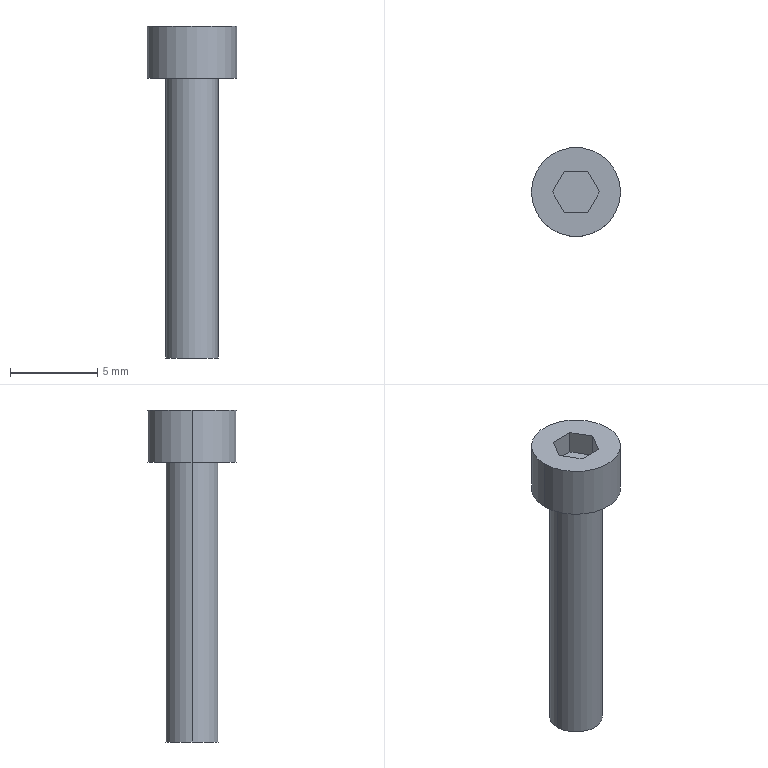Part | SolidWorks | features BaseBody 1 | 1 solid | 14 faces | box 5.1 x 5.1 x 19 mm | volume 167.99 mm3 | plane 10 | cylinder 4 | commonest cylinder face diameters 3 x2 5.1 x2
STEP:
#1=CARTESIAN_POINT('',(1.5,0.,-16.));
#2=VERTEX_POINT('',#1);
#3=CARTESIAN_POINT('',(-1.5,0.,-16.));
#4=VERTEX_POINT('',#3);
#5=CARTESIAN_POINT('',(0.,0.,-16.));
#6=DIRECTION('',(0.,0.,1.));
#7=DIRECTION('',(1.,0.,0.));
#8=AXIS2_PLACEMENT_3D('',#5,#6,#7);
#9=CIRCLE('',#8,1.5);
#10=EDGE_CURVE('',#2,#4,#9,.T.);
#11=ORIENTED_EDGE('',*,*,#10,.T.);
#12=CARTESIAN_POINT('',(-1.5,0.,0.));
#13=VERTEX_POINT('',#12);
#14=CARTESIAN_POINT('',(-1.5,0.,-16.));
#15=DIRECTION('',(0.,0.,1.));
#16=VECTOR('',#15,1000.);
#17=LINE('',#14,#16);
#18=EDGE_CURVE('',#4,#13,#17,.T.);
#19=ORIENTED_EDGE('',*,*,#18,.T.);
#20=CARTESIAN_POINT('',(1.5,0.,0.));
#21=VERTEX_POINT('',#20);
#22=CARTESIAN_POINT('',(0.,0.,0.));
#23=DIRECTION('',(0.,0.,-1.));
#24=DIRECTION('',(1.,0.,0.));
#25=AXIS2_PLACEMENT_3D('',#22,#23,#24);
#26=CIRCLE('',#25,1.5);
#27=EDGE_CURVE('',#13,#21,#26,.T.);
#28=ORIENTED_EDGE('',*,*,#27,.T.);
#29=CARTESIAN_POINT('',(1.5,0.,-16.));
#30=DIRECTION('',(0.,0.,1.));
#31=VECTOR('',#30,1000.);
#32=LINE('',#29,#31);
#33=EDGE_CURVE('',#2,#21,#32,.T.);
#34=ORIENTED_EDGE('',*,*,#33,.F.);
#35=EDGE_LOOP('',(#11,#19,#28,#34));
#36=FACE_OUTER_BOUND('',#35,.T.);
#37=CARTESIAN_POINT('',(0.,0.,-16.));
#38=DIRECTION('',(0.,0.,1.));
#39=DIRECTION('',(1.,0.,0.));
#40=AXIS2_PLACEMENT_3D('',#37,#38,#39);
#41=CYLINDRICAL_SURFACE('',#40,1.5);
#42=ADVANCED_FACE('',(#36),#41,.T.);
#43=CARTESIAN_POINT('',(2.55,0.,0.));
#44=VERTEX_POINT('',#43);
#45=CARTESIAN_POINT('',(-2.55,0.,0.));
#46=VERTEX_POINT('',#45);
#47=CARTESIAN_POINT('',(0.,0.,0.));
#48=DIRECTION('',(0.,0.,1.));
#49=DIRECTION('',(1.,0.,0.));
#50=AXIS2_PLACEMENT_3D('',#47,#48,#49);
#51=CIRCLE('',#50,2.55);
#52=EDGE_CURVE('',#44,#46,#51,.T.);
#53=ORIENTED_EDGE('',*,*,#52,.T.);
#54=CARTESIAN_POINT('',(-2.55,0.,3.));
#55=VERTEX_POINT('',#54);
#56=CARTESIAN_POINT('',(-2.55,0.,0.));
#57=DIRECTION('',(0.,0.,1.));
#58=VECTOR('',#57,1000.);
#59=LINE('',#56,#58);
#60=EDGE_CURVE('',#46,#55,#59,.T.);
#61=ORIENTED_EDGE('',*,*,#60,.T.);
#62=CARTESIAN_POINT('',(2.55,0.,3.));
#63=VERTEX_POINT('',#62);
#64=CARTESIAN_POINT('',(0.,0.,3.));
#65=DIRECTION('',(0.,0.,-1.));
#66=DIRECTION('',(1.,0.,0.));
#67=AXIS2_PLACEMENT_3D('',#64,#65,#66);
#68=CIRCLE('',#67,2.55);
#69=EDGE_CURVE('',#55,#63,#68,.T.);
#70=ORIENTED_EDGE('',*,*,#69,.T.);
#71=CARTESIAN_POINT('',(2.55,0.,0.));
#72=DIRECTION('',(0.,0.,1.));
#73=VECTOR('',#72,1000.);
#74=LINE('',#71,#73);
#75=EDGE_CURVE('',#44,#63,#74,.T.);
#76=ORIENTED_EDGE('',*,*,#75,.F.);
#77=EDGE_LOOP('',(#53,#61,#70,#76));
#78=FACE_OUTER_BOUND('',#77,.T.);
#79=CARTESIAN_POINT('',(0.,0.,0.));
#80=DIRECTION('',(0.,0.,1.));
#81=DIRECTION('',(1.,0.,0.));
#82=AXIS2_PLACEMENT_3D('',#79,#80,#81);
#83=CYLINDRICAL_SURFACE('',#82,2.55);
#84=ADVANCED_FACE('',(#78),#83,.T.);
#85=ORIENTED_EDGE('',*,*,#18,.F.);
#86=CARTESIAN_POINT('',(0.,0.,-16.));
#87=DIRECTION('',(0.,0.,1.));
#88=DIRECTION('',(1.,0.,0.));
#89=AXIS2_PLACEMENT_3D('',#86,#87,#88);
#90=CIRCLE('',#89,1.5);
#91=EDGE_CURVE('',#4,#2,#90,.T.);
#92=ORIENTED_EDGE('',*,*,#91,.T.);
#93=ORIENTED_EDGE('',*,*,#33,.T.);
#94=CARTESIAN_POINT('',(0.,0.,0.));
#95=DIRECTION('',(0.,0.,-1.));
#96=DIRECTION('',(1.,0.,0.));
#97=AXIS2_PLACEMENT_3D('',#94,#95,#96);
#98=CIRCLE('',#97,1.5);
#99=EDGE_CURVE('',#21,#13,#98,.T.);
#100=ORIENTED_EDGE('',*,*,#99,.T.);
#101=EDGE_LOOP('',(#85,#92,#93,#100));
#102=FACE_OUTER_BOUND('',#101,.T.);
#103=CARTESIAN_POINT('',(0.,0.,-16.));
#104=DIRECTION('',(0.,0.,1.));
#105=DIRECTION('',(1.,0.,0.));
#106=AXIS2_PLACEMENT_3D('',#103,#104,#105);
#107=CYLINDRICAL_SURFACE('',#106,1.5);
#108=ADVANCED_FACE('',(#102),#107,.T.);
#109=ORIENTED_EDGE('',*,*,#10,.F.);
#110=ORIENTED_EDGE('',*,*,#91,.F.);
#111=EDGE_LOOP('',(#109,#110));
#112=FACE_OUTER_BOUND('',#111,.T.);
#113=CARTESIAN_POINT('',(0.,0.,-16.));
#114=DIRECTION('',(0.,0.,1.));
#115=DIRECTION('',(1.,0.,0.));
#116=AXIS2_PLACEMENT_3D('',#113,#114,#115);
#117=PLANE('',#116);
#118=ADVANCED_FACE('',(#112),#117,.F.);
#119=ORIENTED_EDGE('',*,*,#99,.F.);
#120=ORIENTED_EDGE('',*,*,#27,.F.);
#121=EDGE_LOOP('',(#119,#120));
#122=FACE_BOUND('',#121,.T.);
#123=ORIENTED_EDGE('',*,*,#52,.F.);
#124=CARTESIAN_POINT('',(0.,0.,0.));
#125=DIRECTION('',(0.,0.,1.));
#126=DIRECTION('',(1.,0.,0.));
#127=AXIS2_PLACEMENT_3D('',#124,#125,#126);
#128=CIRCLE('',#127,2.55);
#129=EDGE_CURVE('',#46,#44,#128,.T.);
#130=ORIENTED_EDGE('',*,*,#129,.F.);
#131=EDGE_LOOP('',(#123,#130));
#132=FACE_OUTER_BOUND('',#131,.T.);
#133=CARTESIAN_POINT('',(0.,0.,0.));
#134=DIRECTION('',(0.,0.,1.));
#135=DIRECTION('',(1.,0.,0.));
#136=AXIS2_PLACEMENT_3D('',#133,#134,#135);
#137=PLANE('',#136);
#138=ADVANCED_FACE('',(#122,#132),#137,.F.);
#139=ORIENTED_EDGE('',*,*,#60,.F.);
#140=ORIENTED_EDGE('',*,*,#129,.T.);
#141=ORIENTED_EDGE('',*,*,#75,.T.);
#142=CARTESIAN_POINT('',(0.,0.,3.));
#143=DIRECTION('',(0.,0.,-1.));
#144=DIRECTION('',(1.,0.,0.));
#145=AXIS2_PLACEMENT_3D('',#142,#143,#144);
#146=CIRCLE('',#145,2.55);
#147=EDGE_CURVE('',#63,#55,#146,.T.);
#148=ORIENTED_EDGE('',*,*,#147,.T.);
#149=EDGE_LOOP('',(#139,#140,#141,#148));
#150=FACE_OUTER_BOUND('',#149,.T.);
#151=CARTESIAN_POINT('',(0.,0.,0.));
#152=DIRECTION('',(0.,0.,1.));
#153=DIRECTION('',(1.,0.,0.));
#154=AXIS2_PLACEMENT_3D('',#151,#152,#153);
#155=CYLINDRICAL_SURFACE('',#154,2.55);
#156=ADVANCED_FACE('',(#150),#155,.T.);
#157=CARTESIAN_POINT('',(-0.675,-1.169,3.));
#158=VERTEX_POINT('',#157);
#159=CARTESIAN_POINT('',(-1.35,0.,3.));
#160=VERTEX_POINT('',#159);
#161=CARTESIAN_POINT('',(-0.675,-1.169,3.));
#162=DIRECTION('',(-0.5,0.866,0.));
#163=VECTOR('',#162,1000.);
#164=LINE('',#161,#163);
#165=EDGE_CURVE('',#158,#160,#164,.T.);
#166=ORIENTED_EDGE('',*,*,#165,.T.);
#167=CARTESIAN_POINT('',(-0.675,1.169,3.));
#168=VERTEX_POINT('',#167);
#169=CARTESIAN_POINT('',(-1.35,0.,3.));
#170=DIRECTION('',(0.5,0.866,0.));
#171=VECTOR('',#170,1000.);
#172=LINE('',#169,#171);
#173=EDGE_CURVE('',#160,#168,#172,.T.);
#174=ORIENTED_EDGE('',*,*,#173,.T.);
#175=CARTESIAN_POINT('',(0.675,1.169,3.));
#176=VERTEX_POINT('',#175);
#177=CARTESIAN_POINT('',(0.,1.169,3.));
#178=DIRECTION('',(1.,0.,0.));
#179=VECTOR('',#178,1000.);
#180=LINE('',#177,#179);
#181=EDGE_CURVE('',#168,#176,#180,.T.);
#182=ORIENTED_EDGE('',*,*,#181,.T.);
#183=CARTESIAN_POINT('',(1.35,0.,3.));
#184=VERTEX_POINT('',#183);
#185=CARTESIAN_POINT('',(0.675,1.169,3.));
#186=DIRECTION('',(0.5,-0.866,0.));
#187=VECTOR('',#186,1000.);
#188=LINE('',#185,#187);
#189=EDGE_CURVE('',#176,#184,#188,.T.);
#190=ORIENTED_EDGE('',*,*,#189,.T.);
#191=CARTESIAN_POINT('',(0.675,-1.169,3.));
#192=VERTEX_POINT('',#191);
#193=CARTESIAN_POINT('',(1.35,0.,3.));
#194=DIRECTION('',(-0.5,-0.866,0.));
#195=VECTOR('',#194,1000.);
#196=LINE('',#193,#195);
#197=EDGE_CURVE('',#184,#192,#196,.T.);
#198=ORIENTED_EDGE('',*,*,#197,.T.);
#199=CARTESIAN_POINT('',(0.,-1.169,3.));
#200=DIRECTION('',(-1.,0.,0.));
#201=VECTOR('',#200,1000.);
#202=LINE('',#199,#201);
#203=EDGE_CURVE('',#192,#158,#202,.T.);
#204=ORIENTED_EDGE('',*,*,#203,.T.);
#205=EDGE_LOOP('',(#166,#174,#182,#190,#198,#204));
#206=FACE_BOUND('',#205,.T.);
#207=ORIENTED_EDGE('',*,*,#147,.F.);
#208=ORIENTED_EDGE('',*,*,#69,.F.);
#209=EDGE_LOOP('',(#207,#208));
#210=FACE_OUTER_BOUND('',#209,.T.);
#211=CARTESIAN_POINT('',(0.,0.,3.));
#212=DIRECTION('',(0.,0.,1.));
#213=DIRECTION('',(1.,0.,0.));
#214=AXIS2_PLACEMENT_3D('',#211,#212,#213);
#215=PLANE('',#214);
#216=ADVANCED_FACE('',(#206,#210),#215,.T.);
#217=ORIENTED_EDGE('',*,*,#173,.F.);
#218=CARTESIAN_POINT('',(-1.35,0.,1.65));
#219=VERTEX_POINT('',#218);
#220=CARTESIAN_POINT('',(-1.35,0.,1.65));
#221=DIRECTION('',(0.,0.,-1.));
#222=VECTOR('',#221,1000.);
#223=LINE('',#220,#222);
#224=EDGE_CURVE('',#160,#219,#223,.T.);
#225=ORIENTED_EDGE('',*,*,#224,.T.);
#226=CARTESIAN_POINT('',(-0.675,1.169,1.65));
#227=VERTEX_POINT('',#226);
#228=CARTESIAN_POINT('',(-0.675,1.169,1.65));
#229=DIRECTION('',(0.5,0.866,0.));
#230=VECTOR('',#229,1000.);
#231=LINE('',#228,#230);
#232=EDGE_CURVE('',#219,#227,#231,.T.);
#233=ORIENTED_EDGE('',*,*,#232,.T.);
#234=CARTESIAN_POINT('',(-0.675,1.169,1.65));
#235=DIRECTION('',(0.,0.,1.));
#236=VECTOR('',#235,1000.);
#237=LINE('',#234,#236);
#238=EDGE_CURVE('',#227,#168,#237,.T.);
#239=ORIENTED_EDGE('',*,*,#238,.T.);
#240=EDGE_LOOP('',(#217,#225,#233,#239));
#241=FACE_OUTER_BOUND('',#240,.T.);
#242=CARTESIAN_POINT('',(-0.675,1.169,1.65));
#243=DIRECTION('',(0.866,-0.5,0.));
#244=DIRECTION('',(0.5,0.866,0.));
#245=AXIS2_PLACEMENT_3D('',#242,#243,#244);
#246=PLANE('',#245);
#247=ADVANCED_FACE('',(#241),#246,.T.);
#248=ORIENTED_EDGE('',*,*,#165,.F.);
#249=CARTESIAN_POINT('',(-0.675,-1.169,1.65));
#250=VERTEX_POINT('',#249);
#251=CARTESIAN_POINT('',(-0.675,-1.169,1.65));
#252=DIRECTION('',(0.,0.,-1.));
#253=VECTOR('',#252,1000.);
#254=LINE('',#251,#253);
#255=EDGE_CURVE('',#158,#250,#254,.T.);
#256=ORIENTED_EDGE('',*,*,#255,.T.);
#257=CARTESIAN_POINT('',(-1.35,0.,1.65));
#258=DIRECTION('',(-0.5,0.866,0.));
#259=VECTOR('',#258,1000.);
#260=LINE('',#257,#259);
#261=EDGE_CURVE('',#250,#219,#260,.T.);
#262=ORIENTED_EDGE('',*,*,#261,.T.);
#263=ORIENTED_EDGE('',*,*,#224,.F.);
#264=EDGE_LOOP('',(#248,#256,#262,#263));
#265=FACE_OUTER_BOUND('',#264,.T.);
#266=CARTESIAN_POINT('',(-1.35,0.,1.65));
#267=DIRECTION('',(0.866,0.5,0.));
#268=DIRECTION('',(-0.5,0.866,0.));
#269=AXIS2_PLACEMENT_3D('',#266,#267,#268);
#270=PLANE('',#269);
#271=ADVANCED_FACE('',(#265),#270,.T.);
#272=ORIENTED_EDGE('',*,*,#203,.F.);
#273=CARTESIAN_POINT('',(0.675,-1.169,1.65));
#274=VERTEX_POINT('',#273);
#275=CARTESIAN_POINT('',(0.675,-1.169,1.65));
#276=DIRECTION('',(0.,0.,-1.));
#277=VECTOR('',#276,1000.);
#278=LINE('',#275,#277);
#279=EDGE_CURVE('',#192,#274,#278,.T.);
#280=ORIENTED_EDGE('',*,*,#279,.T.);
#281=CARTESIAN_POINT('',(-0.675,-1.169,1.65));
#282=DIRECTION('',(-1.,0.,0.));
#283=VECTOR('',#282,1000.);
#284=LINE('',#281,#283);
#285=EDGE_CURVE('',#274,#250,#284,.T.);
#286=ORIENTED_EDGE('',*,*,#285,.T.);
#287=ORIENTED_EDGE('',*,*,#255,.F.);
#288=EDGE_LOOP('',(#272,#280,#286,#287));
#289=FACE_OUTER_BOUND('',#288,.T.);
#290=CARTESIAN_POINT('',(-0.675,-1.169,1.65));
#291=DIRECTION('',(0.,1.,0.));
#292=DIRECTION('',(-1.,0.,0.));
#293=AXIS2_PLACEMENT_3D('',#290,#291,#292);
#294=PLANE('',#293);
#295=ADVANCED_FACE('',(#289),#294,.T.);
#296=ORIENTED_EDGE('',*,*,#197,.F.);
#297=CARTESIAN_POINT('',(1.35,0.,1.65));
#298=VERTEX_POINT('',#297);
#299=CARTESIAN_POINT('',(1.35,0.,1.65));
#300=DIRECTION('',(0.,0.,-1.));
#301=VECTOR('',#300,1000.);
#302=LINE('',#299,#301);
#303=EDGE_CURVE('',#184,#298,#302,.T.);
#304=ORIENTED_EDGE('',*,*,#303,.T.);
#305=CARTESIAN_POINT('',(0.675,-1.169,1.65));
#306=DIRECTION('',(-0.5,-0.866,0.));
#307=VECTOR('',#306,1000.);
#308=LINE('',#305,#307);
#309=EDGE_CURVE('',#298,#274,#308,.T.);
#310=ORIENTED_EDGE('',*,*,#309,.T.);
#311=ORIENTED_EDGE('',*,*,#279,.F.);
#312=EDGE_LOOP('',(#296,#304,#310,#311));
#313=FACE_OUTER_BOUND('',#312,.T.);
#314=CARTESIAN_POINT('',(0.675,-1.169,1.65));
#315=DIRECTION('',(-0.866,0.5,0.));
#316=DIRECTION('',(-0.5,-0.866,0.));
#317=AXIS2_PLACEMENT_3D('',#314,#315,#316);
#318=PLANE('',#317);
#319=ADVANCED_FACE('',(#313),#318,.T.);
#320=ORIENTED_EDGE('',*,*,#189,.F.);
#321=CARTESIAN_POINT('',(0.675,1.169,1.65));
#322=VERTEX_POINT('',#321);
#323=CARTESIAN_POINT('',(0.675,1.169,1.65));
#324=DIRECTION('',(0.,0.,-1.));
#325=VECTOR('',#324,1000.);
#326=LINE('',#323,#325);
#327=EDGE_CURVE('',#176,#322,#326,.T.);
#328=ORIENTED_EDGE('',*,*,#327,.T.);
#329=CARTESIAN_POINT('',(1.35,0.,1.65));
#330=DIRECTION('',(0.5,-0.866,0.));
#331=VECTOR('',#330,1000.);
#332=LINE('',#329,#331);
#333=EDGE_CURVE('',#322,#298,#332,.T.);
#334=ORIENTED_EDGE('',*,*,#333,.T.);
#335=ORIENTED_EDGE('',*,*,#303,.F.);
#336=EDGE_LOOP('',(#320,#328,#334,#335));
#337=FACE_OUTER_BOUND('',#336,.T.);
#338=CARTESIAN_POINT('',(1.35,0.,1.65));
#339=DIRECTION('',(-0.866,-0.5,0.));
#340=DIRECTION('',(0.5,-0.866,0.));
#341=AXIS2_PLACEMENT_3D('',#338,#339,#340);
#342=PLANE('',#341);
#343=ADVANCED_FACE('',(#337),#342,.T.);
#344=ORIENTED_EDGE('',*,*,#181,.F.);
#345=ORIENTED_EDGE('',*,*,#238,.F.);
#346=CARTESIAN_POINT('',(0.675,1.169,1.65));
#347=DIRECTION('',(1.,0.,0.));
#348=VECTOR('',#347,1000.);
#349=LINE('',#346,#348);
#350=EDGE_CURVE('',#227,#322,#349,.T.);
#351=ORIENTED_EDGE('',*,*,#350,.T.);
#352=ORIENTED_EDGE('',*,*,#327,.F.);
#353=EDGE_LOOP('',(#344,#345,#351,#352));
#354=FACE_OUTER_BOUND('',#353,.T.);
#355=CARTESIAN_POINT('',(0.675,1.169,1.65));
#356=DIRECTION('',(0.,-1.,0.));
#357=DIRECTION('',(0.,0.,-1.));
#358=AXIS2_PLACEMENT_3D('',#355,#356,#357);
#359=PLANE('',#358);
#360=ADVANCED_FACE('',(#354),#359,.T.);
#361=ORIENTED_EDGE('',*,*,#285,.F.);
#362=ORIENTED_EDGE('',*,*,#309,.F.);
#363=ORIENTED_EDGE('',*,*,#333,.F.);
#364=ORIENTED_EDGE('',*,*,#350,.F.);
#365=ORIENTED_EDGE('',*,*,#232,.F.);
#366=ORIENTED_EDGE('',*,*,#261,.F.);
#367=EDGE_LOOP('',(#361,#362,#363,#364,#365,#366));
#368=FACE_OUTER_BOUND('',#367,.T.);
#369=CARTESIAN_POINT('',(0.,0.,1.65));
#370=DIRECTION('',(0.,0.,1.));
#371=DIRECTION('',(1.,0.,0.));
#372=AXIS2_PLACEMENT_3D('',#369,#370,#371);
#373=PLANE('',#372);
#374=ADVANCED_FACE('',(#368),#373,.T.);
#375=CLOSED_SHELL('',(#42,#84,#108,#118,#138,#156,#216,#247,#271,#295,#319,#343,#360,#374));
#376=MANIFOLD_SOLID_BREP('',#375);
#377=CARTESIAN_POINT('',(0.,0.,0.));
#378=DIRECTION('',(0.,0.,1.));
#379=DIRECTION('',(1.,0.,0.));
#380=AXIS2_PLACEMENT_3D('',#377,#378,#379);
#381=(LENGTH_UNIT()NAMED_UNIT(*)SI_UNIT(.MILLI.,.METRE.));
#382=UNCERTAINTY_MEASURE_WITH_UNIT(LENGTH_MEASURE(0.00001),#381,'','');
#383=(NAMED_UNIT(*)PLANE_ANGLE_UNIT()SI_UNIT($,.RADIAN.));
#384=(NAMED_UNIT(*)SI_UNIT($,.STERADIAN.)SOLID_ANGLE_UNIT());
#385=(GEOMETRIC_REPRESENTATION_CONTEXT(3)GLOBAL_UNCERTAINTY_ASSIGNED_CONTEXT((#382))GLOBAL_UNIT_ASSIGNED_CONTEXT((#381,#383,#384))REPRESENTATION_CONTEXT('',''));
#386=ADVANCED_BREP_SHAPE_REPRESENTATION('',(#376,#380),#385);